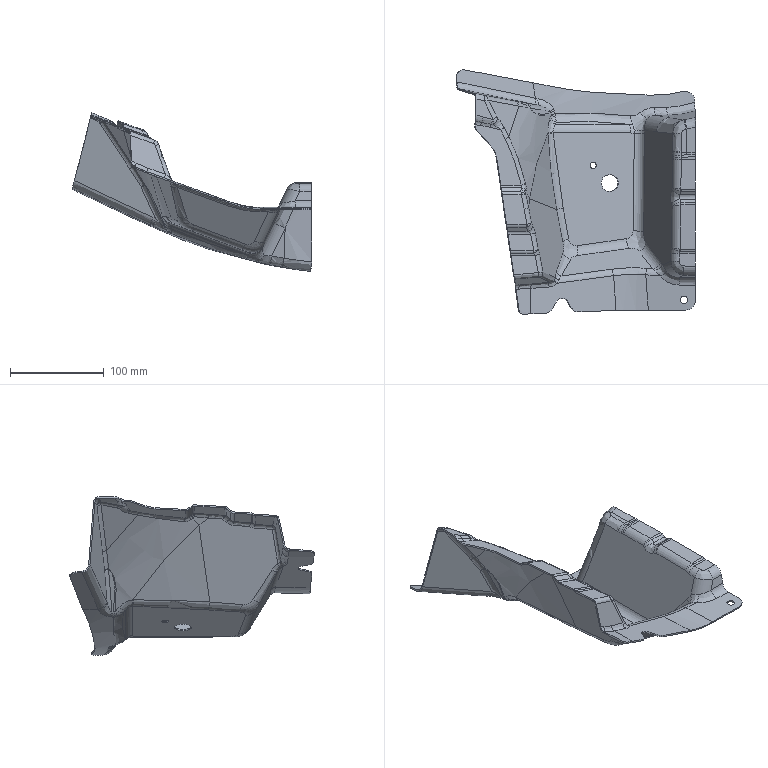Part | 1 solid | 393 faces | box 255.436 x 260.625 x 168.935 mm | volume 122480 mm3 | spline 267 | cylinder 81 | plane 39 | other 6 | commonest cylinder face diameters 10 x11 20 x9 17 x7 7 x6 13 x5 18 x3